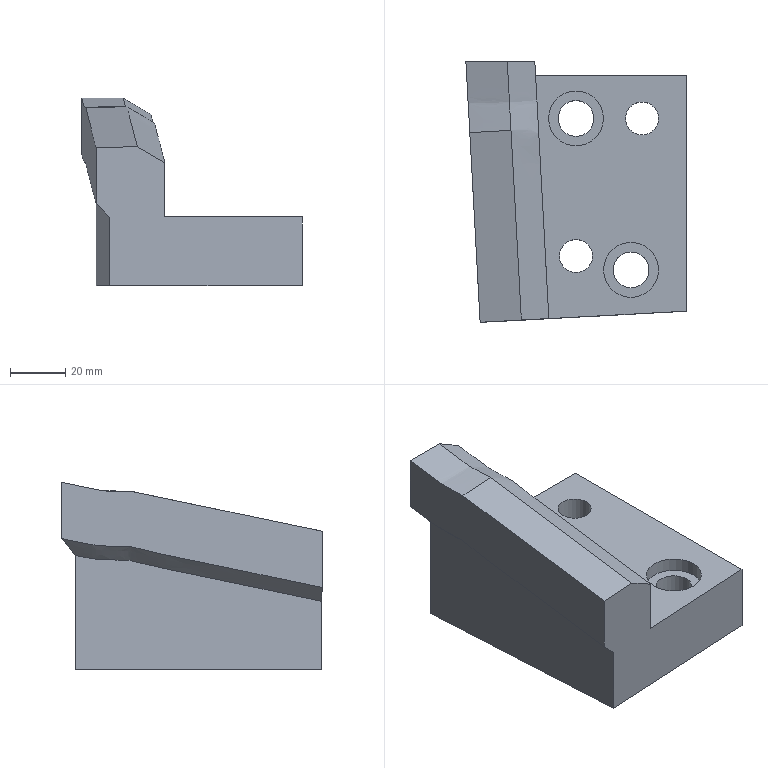Part | NX | features solid 2 | 1 solid | 22 faces | box 80 x 94.651 x 68.104 mm | volume 215629 mm3 | plane 9 | spline 7 | cylinder 6 | commonest cylinder face diameters 12 x2 13 x2 20 x2